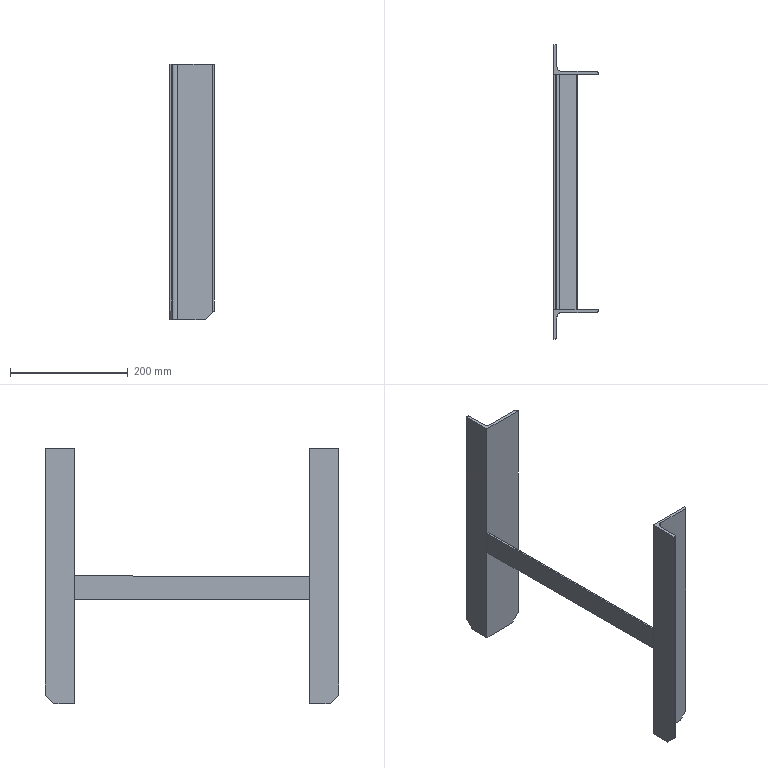Part | SolidWorks | 3 solids | 37 faces | box 75 x 500 x 435 mm | volume 652572 mm3 | plane 28 | cylinder 9 | commonest cylinder face diameters 5.333 x4 2.667 x2 16 x2 10 x1
STEP:
#1=CARTESIAN_POINT('',(75.,0.,-202.5));
#2=VERTEX_POINT('',#1);
#3=CARTESIAN_POINT('',(60.,0.,-217.5));
#4=VERTEX_POINT('',#3);
#5=CARTESIAN_POINT('',(60.,0.,-217.5));
#6=DIRECTION('',(-0.7071,0.,-0.7071));
#7=VECTOR('',#6,1000.);
#8=LINE('',#5,#7);
#9=EDGE_CURVE('',#2,#4,#8,.T.);
#10=ORIENTED_EDGE('',*,*,#9,.F.);
#11=CARTESIAN_POINT('',(75.,0.,217.5));
#12=VERTEX_POINT('',#11);
#13=CARTESIAN_POINT('',(75.,0.,-217.5));
#14=DIRECTION('',(0.,0.,1.));
#15=VECTOR('',#14,1000.);
#16=LINE('',#13,#15);
#17=EDGE_CURVE('',#2,#12,#16,.T.);
#18=ORIENTED_EDGE('',*,*,#17,.T.);
#19=CARTESIAN_POINT('',(0.,0.,217.5));
#20=VERTEX_POINT('',#19);
#21=CARTESIAN_POINT('',(0.,0.,217.5));
#22=DIRECTION('',(-1.,0.,0.));
#23=VECTOR('',#22,1000.);
#24=LINE('',#21,#23);
#25=EDGE_CURVE('',#12,#20,#24,.T.);
#26=ORIENTED_EDGE('',*,*,#25,.T.);
#27=CARTESIAN_POINT('',(0.,0.,-217.5));
#28=VERTEX_POINT('',#27);
#29=CARTESIAN_POINT('',(0.,0.,-217.5));
#30=DIRECTION('',(0.,0.,1.));
#31=VECTOR('',#30,1000.);
#32=LINE('',#29,#31);
#33=EDGE_CURVE('',#28,#20,#32,.T.);
#34=ORIENTED_EDGE('',*,*,#33,.F.);
#35=CARTESIAN_POINT('',(0.,0.,-217.5));
#36=DIRECTION('',(-1.,0.,0.));
#37=VECTOR('',#36,1000.);
#38=LINE('',#35,#37);
#39=EDGE_CURVE('',#4,#28,#38,.T.);
#40=ORIENTED_EDGE('',*,*,#39,.F.);
#41=EDGE_LOOP('',(#10,#18,#26,#34,#40));
#42=FACE_OUTER_BOUND('',#41,.T.);
#43=CARTESIAN_POINT('',(0.,0.,-217.5));
#44=DIRECTION('',(0.,1.,0.));
#45=DIRECTION('',(0.,0.,1.));
#46=AXIS2_PLACEMENT_3D('',#43,#44,#45);
#47=PLANE('',#46);
#48=ADVANCED_FACE('',(#42),#47,.F.);
#49=CARTESIAN_POINT('',(60.,5.,-217.5));
#50=VERTEX_POINT('',#49);
#51=CARTESIAN_POINT('',(60.,-617.801,-217.5));
#52=DIRECTION('',(0.,1.,0.));
#53=VECTOR('',#52,1000.);
#54=LINE('',#51,#53);
#55=EDGE_CURVE('',#4,#50,#54,.T.);
#56=ORIENTED_EDGE('',*,*,#55,.F.);
#57=ORIENTED_EDGE('',*,*,#39,.T.);
#58=CARTESIAN_POINT('',(0.,35.,-217.5));
#59=VERTEX_POINT('',#58);
#60=CARTESIAN_POINT('',(0.,50.,-217.5));
#61=DIRECTION('',(0.,1.,0.));
#62=VECTOR('',#61,1000.);
#63=LINE('',#60,#62);
#64=EDGE_CURVE('',#28,#59,#63,.T.);
#65=ORIENTED_EDGE('',*,*,#64,.T.);
#66=CARTESIAN_POINT('',(5.,35.,-217.5));
#67=VERTEX_POINT('',#66);
#68=CARTESIAN_POINT('',(-555.301,35.,-217.5));
#69=DIRECTION('',(1.,0.,0.));
#70=VECTOR('',#69,1000.);
#71=LINE('',#68,#70);
#72=EDGE_CURVE('',#59,#67,#71,.T.);
#73=ORIENTED_EDGE('',*,*,#72,.T.);
#74=CARTESIAN_POINT('',(5.,13.,-217.5));
#75=VERTEX_POINT('',#74);
#76=CARTESIAN_POINT('',(5.,13.,-217.5));
#77=DIRECTION('',(0.,-1.,0.));
#78=VECTOR('',#77,1000.);
#79=LINE('',#76,#78);
#80=EDGE_CURVE('',#67,#75,#79,.T.);
#81=ORIENTED_EDGE('',*,*,#80,.T.);
#82=CARTESIAN_POINT('',(13.,5.,-217.5));
#83=VERTEX_POINT('',#82);
#84=CARTESIAN_POINT('',(13.,13.,-217.5));
#85=DIRECTION('',(0.,0.,1.));
#86=DIRECTION('',(0.,-1.,0.));
#87=AXIS2_PLACEMENT_3D('',#84,#85,#86);
#88=CIRCLE('',#87,8.);
#89=EDGE_CURVE('',#75,#83,#88,.T.);
#90=ORIENTED_EDGE('',*,*,#89,.T.);
#91=CARTESIAN_POINT('',(72.333,5.,-217.5));
#92=DIRECTION('',(1.,0.,0.));
#93=VECTOR('',#92,1000.);
#94=LINE('',#91,#93);
#95=EDGE_CURVE('',#83,#50,#94,.T.);
#96=ORIENTED_EDGE('',*,*,#95,.T.);
#97=EDGE_LOOP('',(#56,#57,#65,#73,#81,#90,#96));
#98=FACE_OUTER_BOUND('',#97,.T.);
#99=CARTESIAN_POINT('',(72.333,2.333,-217.5));
#100=DIRECTION('',(0.,0.,1.));
#101=DIRECTION('',(0.,-1.,0.));
#102=AXIS2_PLACEMENT_3D('',#99,#100,#101);
#103=PLANE('',#102);
#104=ADVANCED_FACE('',(#98),#103,.F.);
#105=CARTESIAN_POINT('',(0.,50.,-202.5));
#106=VERTEX_POINT('',#105);
#107=CARTESIAN_POINT('',(2.333,50.,-202.5));
#108=VERTEX_POINT('',#107);
#109=CARTESIAN_POINT('',(-555.301,50.,-202.5));
#110=DIRECTION('',(1.,0.,0.));
#111=VECTOR('',#110,1000.);
#112=LINE('',#109,#111);
#113=EDGE_CURVE('',#106,#108,#112,.T.);
#114=ORIENTED_EDGE('',*,*,#113,.F.);
#115=CARTESIAN_POINT('',(0.,50.,217.5));
#116=VERTEX_POINT('',#115);
#117=CARTESIAN_POINT('',(0.,50.,-217.5));
#118=DIRECTION('',(0.,0.,1.));
#119=VECTOR('',#118,1000.);
#120=LINE('',#117,#119);
#121=EDGE_CURVE('',#106,#116,#120,.T.);
#122=ORIENTED_EDGE('',*,*,#121,.T.);
#123=CARTESIAN_POINT('',(2.333,50.,217.5));
#124=VERTEX_POINT('',#123);
#125=CARTESIAN_POINT('',(0.,50.,217.5));
#126=DIRECTION('',(1.,0.,0.));
#127=VECTOR('',#126,1000.);
#128=LINE('',#125,#127);
#129=EDGE_CURVE('',#116,#124,#128,.T.);
#130=ORIENTED_EDGE('',*,*,#129,.T.);
#131=CARTESIAN_POINT('',(2.333,50.,-217.5));
#132=DIRECTION('',(0.,0.,1.));
#133=VECTOR('',#132,1000.);
#134=LINE('',#131,#133);
#135=EDGE_CURVE('',#108,#124,#134,.T.);
#136=ORIENTED_EDGE('',*,*,#135,.F.);
#137=EDGE_LOOP('',(#114,#122,#130,#136));
#138=FACE_OUTER_BOUND('',#137,.T.);
#139=CARTESIAN_POINT('',(0.,50.,-217.5));
#140=DIRECTION('',(0.,-1.,0.));
#141=DIRECTION('',(1.,0.,0.));
#142=AXIS2_PLACEMENT_3D('',#139,#140,#141);
#143=PLANE('',#142);
#144=ADVANCED_FACE('',(#138),#143,.F.);
#145=CARTESIAN_POINT('',(5.,47.333,-205.167));
#146=VERTEX_POINT('',#145);
#147=CARTESIAN_POINT('',(2.333,50.,-202.5));
#148=CARTESIAN_POINT('',(3.895,50.,-202.5));
#149=CARTESIAN_POINT('',(5.,48.895,-203.605));
#150=CARTESIAN_POINT('',(5.,47.333,-205.167));
#151=(BOUNDED_CURVE()B_SPLINE_CURVE(3,(#147,#148,#149,#150),.UNSPECIFIED.,.F.,.F.)B_SPLINE_CURVE_WITH_KNOTS((4,4),(0.,1.571),.UNSPECIFIED.)CURVE()GEOMETRIC_REPRESENTATION_ITEM()RATIONAL_B_SPLINE_CURVE((1.,0.8047,0.8047,1.))REPRESENTATION_ITEM(''));
#152=EDGE_CURVE('',#108,#146,#151,.T.);
#153=ORIENTED_EDGE('',*,*,#152,.F.);
#154=ORIENTED_EDGE('',*,*,#135,.T.);
#155=CARTESIAN_POINT('',(5.,47.333,217.5));
#156=VERTEX_POINT('',#155);
#157=CARTESIAN_POINT('',(2.333,47.333,217.5));
#158=DIRECTION('',(0.,0.,-1.));
#159=DIRECTION('',(0.,1.,0.));
#160=AXIS2_PLACEMENT_3D('',#157,#158,#159);
#161=CIRCLE('',#160,2.667);
#162=EDGE_CURVE('',#124,#156,#161,.T.);
#163=ORIENTED_EDGE('',*,*,#162,.T.);
#164=CARTESIAN_POINT('',(5.,47.333,-217.5));
#165=DIRECTION('',(0.,0.,1.));
#166=VECTOR('',#165,1000.);
#167=LINE('',#164,#166);
#168=EDGE_CURVE('',#146,#156,#167,.T.);
#169=ORIENTED_EDGE('',*,*,#168,.F.);
#170=EDGE_LOOP('',(#153,#154,#163,#169));
#171=FACE_OUTER_BOUND('',#170,.T.);
#172=CARTESIAN_POINT('',(2.333,47.333,-217.5));
#173=DIRECTION('',(0.,0.,1.));
#174=DIRECTION('',(0.,-1.,0.));
#175=AXIS2_PLACEMENT_3D('',#172,#173,#174);
#176=CYLINDRICAL_SURFACE('',#175,2.667);
#177=ADVANCED_FACE('',(#171),#176,.T.);
#178=CARTESIAN_POINT('',(5.,24.,-228.5));
#179=DIRECTION('',(0.,-0.7071,-0.7071));
#180=VECTOR('',#179,1000.);
#181=LINE('',#178,#180);
#182=EDGE_CURVE('',#146,#67,#181,.T.);
#183=ORIENTED_EDGE('',*,*,#182,.F.);
#184=ORIENTED_EDGE('',*,*,#168,.T.);
#185=CARTESIAN_POINT('',(5.,13.,217.5));
#186=VERTEX_POINT('',#185);
#187=CARTESIAN_POINT('',(5.,13.,217.5));
#188=DIRECTION('',(0.,-1.,0.));
#189=VECTOR('',#188,1000.);
#190=LINE('',#187,#189);
#191=EDGE_CURVE('',#156,#186,#190,.T.);
#192=ORIENTED_EDGE('',*,*,#191,.T.);
#193=CARTESIAN_POINT('',(5.,13.,-217.5));
#194=DIRECTION('',(0.,0.,1.));
#195=VECTOR('',#194,1000.);
#196=LINE('',#193,#195);
#197=EDGE_CURVE('',#75,#186,#196,.T.);
#198=ORIENTED_EDGE('',*,*,#197,.F.);
#199=ORIENTED_EDGE('',*,*,#80,.F.);
#200=EDGE_LOOP('',(#183,#184,#192,#198,#199));
#201=FACE_OUTER_BOUND('',#200,.T.);
#202=CARTESIAN_POINT('',(5.,13.,-217.5));
#203=DIRECTION('',(-1.,0.,0.));
#204=DIRECTION('',(0.,-1.,0.));
#205=AXIS2_PLACEMENT_3D('',#202,#203,#204);
#206=PLANE('',#205);
#207=ADVANCED_FACE('',(#201),#206,.F.);
#208=ORIENTED_EDGE('',*,*,#121,.F.);
#209=CARTESIAN_POINT('',(0.,35.,-217.5));
#210=DIRECTION('',(0.,-0.7071,-0.7071));
#211=VECTOR('',#210,1000.);
#212=LINE('',#209,#211);
#213=EDGE_CURVE('',#106,#59,#212,.T.);
#214=ORIENTED_EDGE('',*,*,#213,.T.);
#215=ORIENTED_EDGE('',*,*,#64,.F.);
#216=ORIENTED_EDGE('',*,*,#33,.T.);
#217=CARTESIAN_POINT('',(0.,50.,217.5));
#218=DIRECTION('',(0.,1.,0.));
#219=VECTOR('',#218,1000.);
#220=LINE('',#217,#219);
#221=EDGE_CURVE('',#20,#116,#220,.T.);
#222=ORIENTED_EDGE('',*,*,#221,.T.);
#223=EDGE_LOOP('',(#208,#214,#215,#216,#222));
#224=FACE_OUTER_BOUND('',#223,.T.);
#225=CARTESIAN_POINT('',(0.,50.,-217.5));
#226=DIRECTION('',(1.,0.,0.));
#227=DIRECTION('',(0.,0.,-1.));
#228=AXIS2_PLACEMENT_3D('',#225,#226,#227);
#229=PLANE('',#228);
#230=ADVANCED_FACE('',(#224),#229,.F.);
#231=CARTESIAN_POINT('',(13.,5.,217.5));
#232=VERTEX_POINT('',#231);
#233=CARTESIAN_POINT('',(13.,13.,217.5));
#234=DIRECTION('',(0.,0.,1.));
#235=DIRECTION('',(0.,-1.,0.));
#236=AXIS2_PLACEMENT_3D('',#233,#234,#235);
#237=CIRCLE('',#236,8.);
#238=EDGE_CURVE('',#186,#232,#237,.T.);
#239=ORIENTED_EDGE('',*,*,#238,.T.);
#240=CARTESIAN_POINT('',(13.,5.,-217.5));
#241=DIRECTION('',(0.,0.,1.));
#242=VECTOR('',#241,1000.);
#243=LINE('',#240,#242);
#244=EDGE_CURVE('',#83,#232,#243,.T.);
#245=ORIENTED_EDGE('',*,*,#244,.F.);
#246=ORIENTED_EDGE('',*,*,#89,.F.);
#247=ORIENTED_EDGE('',*,*,#197,.T.);
#248=EDGE_LOOP('',(#239,#245,#246,#247));
#249=FACE_OUTER_BOUND('',#248,.T.);
#250=CARTESIAN_POINT('',(13.,13.,-217.5));
#251=DIRECTION('',(0.,0.,1.));
#252=DIRECTION('',(0.,-1.,0.));
#253=AXIS2_PLACEMENT_3D('',#250,#251,#252);
#254=CYLINDRICAL_SURFACE('',#253,8.);
#255=ADVANCED_FACE('',(#249),#254,.F.);
#256=CARTESIAN_POINT('',(72.333,5.,-205.167));
#257=VERTEX_POINT('',#256);
#258=CARTESIAN_POINT('',(72.333,5.,217.5));
#259=VERTEX_POINT('',#258);
#260=CARTESIAN_POINT('',(72.333,5.,-217.5));
#261=DIRECTION('',(0.,0.,1.));
#262=VECTOR('',#261,1000.);
#263=LINE('',#260,#262);
#264=EDGE_CURVE('',#257,#259,#263,.T.);
#265=ORIENTED_EDGE('',*,*,#264,.F.);
#266=CARTESIAN_POINT('',(66.167,5.,-211.333));
#267=DIRECTION('',(-0.7071,0.,-0.7071));
#268=VECTOR('',#267,1000.);
#269=LINE('',#266,#268);
#270=EDGE_CURVE('',#257,#50,#269,.T.);
#271=ORIENTED_EDGE('',*,*,#270,.T.);
#272=ORIENTED_EDGE('',*,*,#95,.F.);
#273=ORIENTED_EDGE('',*,*,#244,.T.);
#274=CARTESIAN_POINT('',(72.333,5.,217.5));
#275=DIRECTION('',(1.,0.,0.));
#276=VECTOR('',#275,1000.);
#277=LINE('',#274,#276);
#278=EDGE_CURVE('',#232,#259,#277,.T.);
#279=ORIENTED_EDGE('',*,*,#278,.T.);
#280=EDGE_LOOP('',(#265,#271,#272,#273,#279));
#281=FACE_OUTER_BOUND('',#280,.T.);
#282=CARTESIAN_POINT('',(72.333,5.,-217.5));
#283=DIRECTION('',(0.,-1.,0.));
#284=DIRECTION('',(0.,0.,-1.));
#285=AXIS2_PLACEMENT_3D('',#282,#283,#284);
#286=PLANE('',#285);
#287=ADVANCED_FACE('',(#281),#286,.F.);
#288=CARTESIAN_POINT('',(75.,2.333,-202.5));
#289=VERTEX_POINT('',#288);
#290=CARTESIAN_POINT('',(75.,2.333,217.5));
#291=VERTEX_POINT('',#290);
#292=CARTESIAN_POINT('',(75.,2.333,-217.5));
#293=DIRECTION('',(0.,0.,1.));
#294=VECTOR('',#293,1000.);
#295=LINE('',#292,#294);
#296=EDGE_CURVE('',#289,#291,#295,.T.);
#297=ORIENTED_EDGE('',*,*,#296,.F.);
#298=CARTESIAN_POINT('',(75.,2.333,-202.5));
#299=CARTESIAN_POINT('',(75.,3.895,-202.5));
#300=CARTESIAN_POINT('',(73.895,5.,-203.605));
#301=CARTESIAN_POINT('',(72.333,5.,-205.167));
#302=(BOUNDED_CURVE()B_SPLINE_CURVE(3,(#298,#299,#300,#301),.UNSPECIFIED.,.F.,.T.)B_SPLINE_CURVE_WITH_KNOTS((4,4),(0.,1.571),.UNSPECIFIED.)CURVE()GEOMETRIC_REPRESENTATION_ITEM()RATIONAL_B_SPLINE_CURVE((1.,0.8047,0.8047,1.))REPRESENTATION_ITEM(''));
#303=EDGE_CURVE('',#289,#257,#302,.T.);
#304=ORIENTED_EDGE('',*,*,#303,.T.);
#305=ORIENTED_EDGE('',*,*,#264,.T.);
#306=CARTESIAN_POINT('',(72.333,2.333,217.5));
#307=DIRECTION('',(0.,0.,-1.));
#308=DIRECTION('',(0.,-1.,0.));
#309=AXIS2_PLACEMENT_3D('',#306,#307,#308);
#310=CIRCLE('',#309,2.667);
#311=EDGE_CURVE('',#259,#291,#310,.T.);
#312=ORIENTED_EDGE('',*,*,#311,.T.);
#313=EDGE_LOOP('',(#297,#304,#305,#312));
#314=FACE_OUTER_BOUND('',#313,.T.);
#315=CARTESIAN_POINT('',(72.333,2.333,-217.5));
#316=DIRECTION('',(0.,0.,1.));
#317=DIRECTION('',(0.,-1.,0.));
#318=AXIS2_PLACEMENT_3D('',#315,#316,#317);
#319=CYLINDRICAL_SURFACE('',#318,2.667);
#320=ADVANCED_FACE('',(#314),#319,.T.);
#321=ORIENTED_EDGE('',*,*,#17,.F.);
#322=CARTESIAN_POINT('',(75.,-617.801,-202.5));
#323=DIRECTION('',(0.,1.,0.));
#324=VECTOR('',#323,1000.);
#325=LINE('',#322,#324);
#326=EDGE_CURVE('',#2,#289,#325,.T.);
#327=ORIENTED_EDGE('',*,*,#326,.T.);
#328=ORIENTED_EDGE('',*,*,#296,.T.);
#329=CARTESIAN_POINT('',(75.,0.,217.5));
#330=DIRECTION('',(0.,-1.,0.));
#331=VECTOR('',#330,1000.);
#332=LINE('',#329,#331);
#333=EDGE_CURVE('',#291,#12,#332,.T.);
#334=ORIENTED_EDGE('',*,*,#333,.T.);
#335=EDGE_LOOP('',(#321,#327,#328,#334));
#336=FACE_OUTER_BOUND('',#335,.T.);
#337=CARTESIAN_POINT('',(75.,0.,-217.5));
#338=DIRECTION('',(-1.,0.,0.));
#339=DIRECTION('',(0.,-1.,0.));
#340=AXIS2_PLACEMENT_3D('',#337,#338,#339);
#341=PLANE('',#340);
#342=ADVANCED_FACE('',(#336),#341,.F.);
#343=ORIENTED_EDGE('',*,*,#221,.F.);
#344=ORIENTED_EDGE('',*,*,#25,.F.);
#345=ORIENTED_EDGE('',*,*,#333,.F.);
#346=ORIENTED_EDGE('',*,*,#311,.F.);
#347=ORIENTED_EDGE('',*,*,#278,.F.);
#348=ORIENTED_EDGE('',*,*,#238,.F.);
#349=ORIENTED_EDGE('',*,*,#191,.F.);
#350=ORIENTED_EDGE('',*,*,#162,.F.);
#351=ORIENTED_EDGE('',*,*,#129,.F.);
#352=EDGE_LOOP('',(#343,#344,#345,#346,#347,#348,#349,#350,#351));
#353=FACE_OUTER_BOUND('',#352,.T.);
#354=CARTESIAN_POINT('',(72.333,2.333,217.5));
#355=DIRECTION('',(0.,0.,1.));
#356=DIRECTION('',(0.,-1.,0.));
#357=AXIS2_PLACEMENT_3D('',#354,#355,#356);
#358=PLANE('',#357);
#359=ADVANCED_FACE('',(#353),#358,.T.);
#360=ORIENTED_EDGE('',*,*,#113,.T.);
#361=ORIENTED_EDGE('',*,*,#152,.T.);
#362=ORIENTED_EDGE('',*,*,#182,.T.);
#363=ORIENTED_EDGE('',*,*,#72,.F.);
#364=ORIENTED_EDGE('',*,*,#213,.F.);
#365=EDGE_LOOP('',(#360,#361,#362,#363,#364));
#366=FACE_OUTER_BOUND('',#365,.T.);
#367=CARTESIAN_POINT('',(-555.301,35.,-217.5));
#368=DIRECTION('',(0.,0.7071,-0.7071));
#369=DIRECTION('',(0.,0.7071,0.7071));
#370=AXIS2_PLACEMENT_3D('',#367,#368,#369);
#371=PLANE('',#370);
#372=ADVANCED_FACE('',(#366),#371,.T.);
#373=ORIENTED_EDGE('',*,*,#270,.F.);
#374=ORIENTED_EDGE('',*,*,#303,.F.);
#375=ORIENTED_EDGE('',*,*,#326,.F.);
#376=ORIENTED_EDGE('',*,*,#9,.T.);
#377=ORIENTED_EDGE('',*,*,#55,.T.);
#378=EDGE_LOOP('',(#373,#374,#375,#376,#377));
#379=FACE_OUTER_BOUND('',#378,.T.);
#380=CARTESIAN_POINT('',(60.,-617.801,-217.5));
#381=DIRECTION('',(-0.7071,0.,0.7071));
#382=DIRECTION('',(0.7071,0.,0.7071));
#383=AXIS2_PLACEMENT_3D('',#380,#381,#382);
#384=PLANE('',#383);
#385=ADVANCED_FACE('',(#379),#384,.F.);
#386=CLOSED_SHELL('',(#48,#104,#144,#177,#207,#230,#255,#287,#320,#342,#359,#372,#385));
#387=MANIFOLD_SOLID_BREP('',#386);
#388=CARTESIAN_POINT('',(75.,-400.,-202.5));
#389=VERTEX_POINT('',#388);
#390=CARTESIAN_POINT('',(60.,-400.,-217.5));
#391=VERTEX_POINT('',#390);
#392=CARTESIAN_POINT('',(60.,-400.,-217.5));
#393=DIRECTION('',(-0.7071,0.,-0.7071));
#394=VECTOR('',#393,1000.);
#395=LINE('',#392,#394);
#396=EDGE_CURVE('',#389,#391,#395,.T.);
#397=ORIENTED_EDGE('',*,*,#396,.T.);
#398=CARTESIAN_POINT('',(0.,-400.,-217.5));
#399=VERTEX_POINT('',#398);
#400=CARTESIAN_POINT('',(0.,-400.,-217.5));
#401=DIRECTION('',(-1.,0.,0.));
#402=VECTOR('',#401,1000.);
#403=LINE('',#400,#402);
#404=EDGE_CURVE('',#391,#399,#403,.T.);
#405=ORIENTED_EDGE('',*,*,#404,.T.);
#406=CARTESIAN_POINT('',(0.,-400.,217.5));
#407=VERTEX_POINT('',#406);
#408=CARTESIAN_POINT('',(0.,-400.,-217.5));
#409=DIRECTION('',(0.,0.,1.));
#410=VECTOR('',#409,1000.);
#411=LINE('',#408,#410);
#412=EDGE_CURVE('',#399,#407,#411,.T.);
#413=ORIENTED_EDGE('',*,*,#412,.T.);
#414=CARTESIAN_POINT('',(75.,-400.,217.5));
#415=VERTEX_POINT('',#414);
#416=CARTESIAN_POINT('',(0.,-400.,217.5));
#417=DIRECTION('',(-1.,0.,0.));
#418=VECTOR('',#417,1000.);
#419=LINE('',#416,#418);
#420=EDGE_CURVE('',#415,#407,#419,.T.);
#421=ORIENTED_EDGE('',*,*,#420,.F.);
#422=CARTESIAN_POINT('',(75.,-400.,-217.5));
#423=DIRECTION('',(0.,0.,1.));
#424=VECTOR('',#423,1000.);
#425=LINE('',#422,#424);
#426=EDGE_CURVE('',#389,#415,#425,.T.);
#427=ORIENTED_EDGE('',*,*,#426,.F.);
#428=EDGE_LOOP('',(#397,#405,#413,#421,#427));
#429=FACE_OUTER_BOUND('',#428,.T.);
#430=CARTESIAN_POINT('',(0.,-400.,-217.5));
#431=DIRECTION('',(0.,-1.,0.));
#432=DIRECTION('',(0.,0.,1.));
#433=AXIS2_PLACEMENT_3D('',#430,#431,#432);
#434=PLANE('',#433);
#435=ADVANCED_FACE('',(#429),#434,.F.);
#436=CARTESIAN_POINT('',(60.,-405.,-217.5));
#437=VERTEX_POINT('',#436);
#438=CARTESIAN_POINT('',(60.,217.801,-217.5));
#439=DIRECTION('',(0.,-1.,0.));
#440=VECTOR('',#439,1000.);
#441=LINE('',#438,#440);
#442=EDGE_CURVE('',#391,#437,#441,.T.);
#443=ORIENTED_EDGE('',*,*,#442,.T.);
#444=CARTESIAN_POINT('',(13.,-405.,-217.5));
#445=VERTEX_POINT('',#444);
#446=CARTESIAN_POINT('',(72.333,-405.,-217.5));
#447=DIRECTION('',(1.,0.,0.));
#448=VECTOR('',#447,1000.);
#449=LINE('',#446,#448);
#450=EDGE_CURVE('',#445,#437,#449,.T.);
#451=ORIENTED_EDGE('',*,*,#450,.F.);
#452=CARTESIAN_POINT('',(5.,-413.,-217.5));
#453=VERTEX_POINT('',#452);
#454=CARTESIAN_POINT('',(13.,-413.,-217.5));
#455=DIRECTION('',(0.,0.,-1.));
#456=DIRECTION('',(0.,1.,0.));
#457=AXIS2_PLACEMENT_3D('',#454,#455,#456);
#458=CIRCLE('',#457,8.);
#459=EDGE_CURVE('',#453,#445,#458,.T.);
#460=ORIENTED_EDGE('',*,*,#459,.F.);
#461=CARTESIAN_POINT('',(5.,-435.,-217.5));
#462=VERTEX_POINT('',#461);
#463=CARTESIAN_POINT('',(5.,-413.,-217.5));
#464=DIRECTION('',(0.,1.,0.));
#465=VECTOR('',#464,1000.);
#466=LINE('',#463,#465);
#467=EDGE_CURVE('',#462,#453,#466,.T.);
#468=ORIENTED_EDGE('',*,*,#467,.F.);
#469=CARTESIAN_POINT('',(0.,-435.,-217.5));
#470=VERTEX_POINT('',#469);
#471=CARTESIAN_POINT('',(-555.301,-435.,-217.5));
#472=DIRECTION('',(1.,0.,0.));
#473=VECTOR('',#472,1000.);
#474=LINE('',#471,#473);
#475=EDGE_CURVE('',#470,#462,#474,.T.);
#476=ORIENTED_EDGE('',*,*,#475,.F.);
#477=CARTESIAN_POINT('',(0.,-450.,-217.5));
#478=DIRECTION('',(0.,-1.,0.));
#479=VECTOR('',#478,1000.);
#480=LINE('',#477,#479);
#481=EDGE_CURVE('',#399,#470,#480,.T.);
#482=ORIENTED_EDGE('',*,*,#481,.F.);
#483=ORIENTED_EDGE('',*,*,#404,.F.);
#484=EDGE_LOOP('',(#443,#451,#460,#468,#476,#482,#483));
#485=FACE_OUTER_BOUND('',#484,.T.);
#486=CARTESIAN_POINT('',(72.333,-402.333,-217.5));
#487=DIRECTION('',(0.,0.,1.));
#488=DIRECTION('',(0.,1.,0.));
#489=AXIS2_PLACEMENT_3D('',#486,#487,#488);
#490=PLANE('',#489);
#491=ADVANCED_FACE('',(#485),#490,.F.);
#492=CARTESIAN_POINT('',(0.,-450.,-202.5));
#493=VERTEX_POINT('',#492);
#494=CARTESIAN_POINT('',(2.333,-450.,-202.5));
#495=VERTEX_POINT('',#494);
#496=CARTESIAN_POINT('',(-555.301,-450.,-202.5));
#497=DIRECTION('',(1.,0.,0.));
#498=VECTOR('',#497,1000.);
#499=LINE('',#496,#498);
#500=EDGE_CURVE('',#493,#495,#499,.T.);
#501=ORIENTED_EDGE('',*,*,#500,.T.);
#502=CARTESIAN_POINT('',(2.333,-450.,217.5));
#503=VERTEX_POINT('',#502);
#504=CARTESIAN_POINT('',(2.333,-450.,-217.5));
#505=DIRECTION('',(0.,0.,1.));
#506=VECTOR('',#505,1000.);
#507=LINE('',#504,#506);
#508=EDGE_CURVE('',#495,#503,#507,.T.);
#509=ORIENTED_EDGE('',*,*,#508,.T.);
#510=CARTESIAN_POINT('',(0.,-450.,217.5));
#511=VERTEX_POINT('',#510);
#512=CARTESIAN_POINT('',(0.,-450.,217.5));
#513=DIRECTION('',(1.,0.,0.));
#514=VECTOR('',#513,1000.);
#515=LINE('',#512,#514);
#516=EDGE_CURVE('',#511,#503,#515,.T.);
#517=ORIENTED_EDGE('',*,*,#516,.F.);
#518=CARTESIAN_POINT('',(0.,-450.,-217.5));
#519=DIRECTION('',(0.,0.,1.));
#520=VECTOR('',#519,1000.);
#521=LINE('',#518,#520);
#522=EDGE_CURVE('',#493,#511,#521,.T.);
#523=ORIENTED_EDGE('',*,*,#522,.F.);
#524=EDGE_LOOP('',(#501,#509,#517,#523));
#525=FACE_OUTER_BOUND('',#524,.T.);
#526=CARTESIAN_POINT('',(0.,-450.,-217.5));
#527=DIRECTION('',(0.,1.,0.));
#528=DIRECTION('',(1.,0.,0.));
#529=AXIS2_PLACEMENT_3D('',#526,#527,#528);
#530=PLANE('',#529);
#531=ADVANCED_FACE('',(#525),#530,.F.);
#532=CARTESIAN_POINT('',(5.,-447.333,-205.167));
#533=VERTEX_POINT('',#532);
#534=CARTESIAN_POINT('',(2.333,-450.,-202.5));
#535=CARTESIAN_POINT('',(3.895,-450.,-202.5));
#536=CARTESIAN_POINT('',(5.,-448.895,-203.605));
#537=CARTESIAN_POINT('',(5.,-447.333,-205.167));
#538=(BOUNDED_CURVE()B_SPLINE_CURVE(3,(#534,#535,#536,#537),.UNSPECIFIED.,.F.,.T.)B_SPLINE_CURVE_WITH_KNOTS((4,4),(0.,1.571),.UNSPECIFIED.)CURVE()GEOMETRIC_REPRESENTATION_ITEM()RATIONAL_B_SPLINE_CURVE((1.,0.8047,0.8047,1.))REPRESENTATION_ITEM(''));
#539=EDGE_CURVE('',#495,#533,#538,.T.);
#540=ORIENTED_EDGE('',*,*,#539,.T.);
#541=CARTESIAN_POINT('',(5.,-447.333,217.5));
#542=VERTEX_POINT('',#541);
#543=CARTESIAN_POINT('',(5.,-447.333,-217.5));
#544=DIRECTION('',(0.,0.,1.));
#545=VECTOR('',#544,1000.);
#546=LINE('',#543,#545);
#547=EDGE_CURVE('',#533,#542,#546,.T.);
#548=ORIENTED_EDGE('',*,*,#547,.T.);
#549=CARTESIAN_POINT('',(2.333,-447.333,217.5));
#550=DIRECTION('',(0.,0.,1.));
#551=DIRECTION('',(0.,-1.,0.));
#552=AXIS2_PLACEMENT_3D('',#549,#550,#551);
#553=CIRCLE('',#552,2.667);
#554=EDGE_CURVE('',#503,#542,#553,.T.);
#555=ORIENTED_EDGE('',*,*,#554,.F.);
#556=ORIENTED_EDGE('',*,*,#508,.F.);
#557=EDGE_LOOP('',(#540,#548,#555,#556));
#558=FACE_OUTER_BOUND('',#557,.T.);
#559=CARTESIAN_POINT('',(2.333,-447.333,-217.5));
#560=DIRECTION('',(0.,0.,1.));
#561=DIRECTION('',(0.,1.,0.));
#562=AXIS2_PLACEMENT_3D('',#559,#560,#561);
#563=CYLINDRICAL_SURFACE('',#562,2.667);
#564=ADVANCED_FACE('',(#558),#563,.T.);
#565=CARTESIAN_POINT('',(5.,-424.,-228.5));
#566=DIRECTION('',(0.,0.7071,-0.7071));
#567=VECTOR('',#566,1000.);
#568=LINE('',#565,#567);
#569=EDGE_CURVE('',#533,#462,#568,.T.);
#570=ORIENTED_EDGE('',*,*,#569,.T.);
#571=ORIENTED_EDGE('',*,*,#467,.T.);
#572=CARTESIAN_POINT('',(5.,-413.,217.5));
#573=VERTEX_POINT('',#572);
#574=CARTESIAN_POINT('',(5.,-413.,-217.5));
#575=DIRECTION('',(0.,0.,1.));
#576=VECTOR('',#575,1000.);
#577=LINE('',#574,#576);
#578=EDGE_CURVE('',#453,#573,#577,.T.);
#579=ORIENTED_EDGE('',*,*,#578,.T.);
#580=CARTESIAN_POINT('',(5.,-413.,217.5));
#581=DIRECTION('',(0.,1.,0.));
#582=VECTOR('',#581,1000.);
#583=LINE('',#580,#582);
#584=EDGE_CURVE('',#542,#573,#583,.T.);
#585=ORIENTED_EDGE('',*,*,#584,.F.);
#586=ORIENTED_EDGE('',*,*,#547,.F.);
#587=EDGE_LOOP('',(#570,#571,#579,#585,#586));
#588=FACE_OUTER_BOUND('',#587,.T.);
#589=CARTESIAN_POINT('',(5.,-413.,-217.5));
#590=DIRECTION('',(-1.,0.,0.));
#591=DIRECTION('',(0.,1.,0.));
#592=AXIS2_PLACEMENT_3D('',#589,#590,#591);
#593=PLANE('',#592);
#594=ADVANCED_FACE('',(#588),#593,.F.);
#595=ORIENTED_EDGE('',*,*,#522,.T.);
#596=CARTESIAN_POINT('',(0.,-450.,217.5));
#597=DIRECTION('',(0.,-1.,0.));
#598=VECTOR('',#597,1000.);
#599=LINE('',#596,#598);
#600=EDGE_CURVE('',#407,#511,#599,.T.);
#601=ORIENTED_EDGE('',*,*,#600,.F.);
#602=ORIENTED_EDGE('',*,*,#412,.F.);
#603=ORIENTED_EDGE('',*,*,#481,.T.);
#604=CARTESIAN_POINT('',(0.,-435.,-217.5));
#605=DIRECTION('',(0.,0.7071,-0.7071));
#606=VECTOR('',#605,1000.);
#607=LINE('',#604,#606);
#608=EDGE_CURVE('',#493,#470,#607,.T.);
#609=ORIENTED_EDGE('',*,*,#608,.F.);
#610=EDGE_LOOP('',(#595,#601,#602,#603,#609));
#611=FACE_OUTER_BOUND('',#610,.T.);
#612=CARTESIAN_POINT('',(0.,-450.,-217.5));
#613=DIRECTION('',(1.,0.,0.));
#614=DIRECTION('',(0.,0.,-1.));
#615=AXIS2_PLACEMENT_3D('',#612,#613,#614);
#616=PLANE('',#615);
#617=ADVANCED_FACE('',(#611),#616,.F.);
#618=CARTESIAN_POINT('',(13.,-405.,217.5));
#619=VERTEX_POINT('',#618);
#620=CARTESIAN_POINT('',(13.,-413.,217.5));
#621=DIRECTION('',(0.,0.,-1.));
#622=DIRECTION('',(0.,1.,0.));
#623=AXIS2_PLACEMENT_3D('',#620,#621,#622);
#624=CIRCLE('',#623,8.);
#625=EDGE_CURVE('',#573,#619,#624,.T.);
#626=ORIENTED_EDGE('',*,*,#625,.F.);
#627=ORIENTED_EDGE('',*,*,#578,.F.);
#628=ORIENTED_EDGE('',*,*,#459,.T.);
#629=CARTESIAN_POINT('',(13.,-405.,-217.5));
#630=DIRECTION('',(0.,0.,1.));
#631=VECTOR('',#630,1000.);
#632=LINE('',#629,#631);
#633=EDGE_CURVE('',#445,#619,#632,.T.);
#634=ORIENTED_EDGE('',*,*,#633,.T.);
#635=EDGE_LOOP('',(#626,#627,#628,#634));
#636=FACE_OUTER_BOUND('',#635,.T.);
#637=CARTESIAN_POINT('',(13.,-413.,-217.5));
#638=DIRECTION('',(0.,0.,1.));
#639=DIRECTION('',(0.,1.,0.));
#640=AXIS2_PLACEMENT_3D('',#637,#638,#639);
#641=CYLINDRICAL_SURFACE('',#640,8.);
#642=ADVANCED_FACE('',(#636),#641,.F.);
#643=CARTESIAN_POINT('',(72.333,-405.,-205.167));
#644=VERTEX_POINT('',#643);
#645=CARTESIAN_POINT('',(72.333,-405.,217.5));
#646=VERTEX_POINT('',#645);
#647=CARTESIAN_POINT('',(72.333,-405.,-217.5));
#648=DIRECTION('',(0.,0.,1.));
#649=VECTOR('',#648,1000.);
#650=LINE('',#647,#649);
#651=EDGE_CURVE('',#644,#646,#650,.T.);
#652=ORIENTED_EDGE('',*,*,#651,.T.);
#653=CARTESIAN_POINT('',(72.333,-405.,217.5));
#654=DIRECTION('',(1.,0.,0.));
#655=VECTOR('',#654,1000.);
#656=LINE('',#653,#655);
#657=EDGE_CURVE('',#619,#646,#656,.T.);
#658=ORIENTED_EDGE('',*,*,#657,.F.);
#659=ORIENTED_EDGE('',*,*,#633,.F.);
#660=ORIENTED_EDGE('',*,*,#450,.T.);
#661=CARTESIAN_POINT('',(66.167,-405.,-211.333));
#662=DIRECTION('',(-0.7071,0.,-0.7071));
#663=VECTOR('',#662,1000.);
#664=LINE('',#661,#663);
#665=EDGE_CURVE('',#644,#437,#664,.T.);
#666=ORIENTED_EDGE('',*,*,#665,.F.);
#667=EDGE_LOOP('',(#652,#658,#659,#660,#666));
#668=FACE_OUTER_BOUND('',#667,.T.);
#669=CARTESIAN_POINT('',(72.333,-405.,-217.5));
#670=DIRECTION('',(0.,1.,0.));
#671=DIRECTION('',(0.,0.,-1.));
#672=AXIS2_PLACEMENT_3D('',#669,#670,#671);
#673=PLANE('',#672);
#674=ADVANCED_FACE('',(#668),#673,.F.);
#675=CARTESIAN_POINT('',(75.,-402.333,-202.5));
#676=VERTEX_POINT('',#675);
#677=CARTESIAN_POINT('',(75.,-402.333,217.5));
#678=VERTEX_POINT('',#677);
#679=CARTESIAN_POINT('',(75.,-402.333,-217.5));
#680=DIRECTION('',(0.,0.,1.));
#681=VECTOR('',#680,1000.);
#682=LINE('',#679,#681);
#683=EDGE_CURVE('',#676,#678,#682,.T.);
#684=ORIENTED_EDGE('',*,*,#683,.T.);
#685=CARTESIAN_POINT('',(72.333,-402.333,217.5));
#686=DIRECTION('',(0.,0.,1.));
#687=DIRECTION('',(0.,1.,0.));
#688=AXIS2_PLACEMENT_3D('',#685,#686,#687);
#689=CIRCLE('',#688,2.667);
#690=EDGE_CURVE('',#646,#678,#689,.T.);
#691=ORIENTED_EDGE('',*,*,#690,.F.);
#692=ORIENTED_EDGE('',*,*,#651,.F.);
#693=CARTESIAN_POINT('',(75.,-402.333,-202.5));
#694=CARTESIAN_POINT('',(75.,-403.895,-202.5));
#695=CARTESIAN_POINT('',(73.895,-405.,-203.605));
#696=CARTESIAN_POINT('',(72.333,-405.,-205.167));
#697=(BOUNDED_CURVE()B_SPLINE_CURVE(3,(#693,#694,#695,#696),.UNSPECIFIED.,.F.,.F.)B_SPLINE_CURVE_WITH_KNOTS((4,4),(0.,1.571),.UNSPECIFIED.)CURVE()GEOMETRIC_REPRESENTATION_ITEM()RATIONAL_B_SPLINE_CURVE((1.,0.8047,0.8047,1.))REPRESENTATION_ITEM(''));
#698=EDGE_CURVE('',#676,#644,#697,.T.);
#699=ORIENTED_EDGE('',*,*,#698,.F.);
#700=EDGE_LOOP('',(#684,#691,#692,#699));
#701=FACE_OUTER_BOUND('',#700,.T.);
#702=CARTESIAN_POINT('',(72.333,-402.333,-217.5));
#703=DIRECTION('',(0.,0.,1.));
#704=DIRECTION('',(0.,1.,0.));
#705=AXIS2_PLACEMENT_3D('',#702,#703,#704);
#706=CYLINDRICAL_SURFACE('',#705,2.667);
#707=ADVANCED_FACE('',(#701),#706,.T.);
#708=ORIENTED_EDGE('',*,*,#426,.T.);
#709=CARTESIAN_POINT('',(75.,-400.,217.5));
#710=DIRECTION('',(0.,1.,0.));
#711=VECTOR('',#710,1000.);
#712=LINE('',#709,#711);
#713=EDGE_CURVE('',#678,#415,#712,.T.);
#714=ORIENTED_EDGE('',*,*,#713,.F.);
#715=ORIENTED_EDGE('',*,*,#683,.F.);
#716=CARTESIAN_POINT('',(75.,217.801,-202.5));
#717=DIRECTION('',(0.,-1.,0.));
#718=VECTOR('',#717,1000.);
#719=LINE('',#716,#718);
#720=EDGE_CURVE('',#389,#676,#719,.T.);
#721=ORIENTED_EDGE('',*,*,#720,.F.);
#722=EDGE_LOOP('',(#708,#714,#715,#721));
#723=FACE_OUTER_BOUND('',#722,.T.);
#724=CARTESIAN_POINT('',(75.,-400.,-217.5));
#725=DIRECTION('',(-1.,0.,0.));
#726=DIRECTION('',(0.,1.,0.));
#727=AXIS2_PLACEMENT_3D('',#724,#725,#726);
#728=PLANE('',#727);
#729=ADVANCED_FACE('',(#723),#728,.F.);
#730=ORIENTED_EDGE('',*,*,#600,.T.);
#731=ORIENTED_EDGE('',*,*,#516,.T.);
#732=ORIENTED_EDGE('',*,*,#554,.T.);
#733=ORIENTED_EDGE('',*,*,#584,.T.);
#734=ORIENTED_EDGE('',*,*,#625,.T.);
#735=ORIENTED_EDGE('',*,*,#657,.T.);
#736=ORIENTED_EDGE('',*,*,#690,.T.);
#737=ORIENTED_EDGE('',*,*,#713,.T.);
#738=ORIENTED_EDGE('',*,*,#420,.T.);
#739=EDGE_LOOP('',(#730,#731,#732,#733,#734,#735,#736,#737,#738));
#740=FACE_OUTER_BOUND('',#739,.T.);
#741=CARTESIAN_POINT('',(72.333,-402.333,217.5));
#742=DIRECTION('',(0.,0.,1.));
#743=DIRECTION('',(0.,1.,0.));
#744=AXIS2_PLACEMENT_3D('',#741,#742,#743);
#745=PLANE('',#744);
#746=ADVANCED_FACE('',(#740),#745,.T.);
#747=ORIENTED_EDGE('',*,*,#500,.F.);
#748=ORIENTED_EDGE('',*,*,#608,.T.);
#749=ORIENTED_EDGE('',*,*,#475,.T.);
#750=ORIENTED_EDGE('',*,*,#569,.F.);
#751=ORIENTED_EDGE('',*,*,#539,.F.);
#752=EDGE_LOOP('',(#747,#748,#749,#750,#751));
#753=FACE_OUTER_BOUND('',#752,.T.);
#754=CARTESIAN_POINT('',(-555.301,-435.,-217.5));
#755=DIRECTION('',(0.,-0.7071,-0.7071));
#756=DIRECTION('',(0.,-0.7071,0.7071));
#757=AXIS2_PLACEMENT_3D('',#754,#755,#756);
#758=PLANE('',#757);
#759=ADVANCED_FACE('',(#753),#758,.T.);
#760=ORIENTED_EDGE('',*,*,#665,.T.);
#761=ORIENTED_EDGE('',*,*,#442,.F.);
#762=ORIENTED_EDGE('',*,*,#396,.F.);
#763=ORIENTED_EDGE('',*,*,#720,.T.);
#764=ORIENTED_EDGE('',*,*,#698,.T.);
#765=EDGE_LOOP('',(#760,#761,#762,#763,#764));
#766=FACE_OUTER_BOUND('',#765,.T.);
#767=CARTESIAN_POINT('',(60.,217.801,-217.5));
#768=DIRECTION('',(-0.7071,0.,0.7071));
#769=DIRECTION('',(0.7071,0.,0.7071));
#770=AXIS2_PLACEMENT_3D('',#767,#768,#769);
#771=PLANE('',#770);
#772=ADVANCED_FACE('',(#766),#771,.F.);
#773=CLOSED_SHELL('',(#435,#491,#531,#564,#594,#617,#642,#674,#707,#729,#746,#759,#772));
#774=MANIFOLD_SOLID_BREP('',#773);
#775=CARTESIAN_POINT('',(0.,0.,-40.));
#776=VERTEX_POINT('',#775);
#777=CARTESIAN_POINT('',(0.,0.,0.));
#778=VERTEX_POINT('',#777);
#779=CARTESIAN_POINT('',(0.,0.,0.));
#780=DIRECTION('',(0.,0.,1.));
#781=VECTOR('',#780,1000.);
#782=LINE('',#779,#781);
#783=EDGE_CURVE('',#776,#778,#782,.T.);
#784=ORIENTED_EDGE('',*,*,#783,.F.);
#785=CARTESIAN_POINT('',(0.,-400.,-40.));
#786=VERTEX_POINT('',#785);
#787=CARTESIAN_POINT('',(0.,-400.,-40.));
#788=DIRECTION('',(0.,1.,0.));
#789=VECTOR('',#788,1000.);
#790=LINE('',#787,#789);
#791=EDGE_CURVE('',#786,#776,#790,.T.);
#792=ORIENTED_EDGE('',*,*,#791,.F.);
#793=CARTESIAN_POINT('',(0.,-400.,0.));
#794=VERTEX_POINT('',#793);
#795=CARTESIAN_POINT('',(0.,-400.,0.));
#796=DIRECTION('',(0.,0.,1.));
#797=VECTOR('',#796,1000.);
#798=LINE('',#795,#797);
#799=EDGE_CURVE('',#786,#794,#798,.T.);
#800=ORIENTED_EDGE('',*,*,#799,.T.);
#801=CARTESIAN_POINT('',(0.,-400.,0.));
#802=DIRECTION('',(0.,1.,0.));
#803=VECTOR('',#802,1000.);
#804=LINE('',#801,#803);
#805=EDGE_CURVE('',#794,#778,#804,.T.);
#806=ORIENTED_EDGE('',*,*,#805,.T.);
#807=EDGE_LOOP('',(#784,#792,#800,#806));
#808=FACE_OUTER_BOUND('',#807,.T.);
#809=CARTESIAN_POINT('',(0.,-400.,0.));
#810=DIRECTION('',(-1.,0.,0.));
#811=DIRECTION('',(0.,0.,1.));
#812=AXIS2_PLACEMENT_3D('',#809,#810,#811);
#813=PLANE('',#812);
#814=ADVANCED_FACE('',(#808),#813,.T.);
#815=CARTESIAN_POINT('',(40.,0.,-40.));
#816=VERTEX_POINT('',#815);
#817=CARTESIAN_POINT('',(0.,0.,-40.));
#818=DIRECTION('',(-1.,0.,0.));
#819=VECTOR('',#818,1000.);
#820=LINE('',#817,#819);
#821=EDGE_CURVE('',#816,#776,#820,.T.);
#822=ORIENTED_EDGE('',*,*,#821,.F.);
#823=CARTESIAN_POINT('',(40.,-400.,-40.));
#824=VERTEX_POINT('',#823);
#825=CARTESIAN_POINT('',(40.,-400.,-40.));
#826=DIRECTION('',(0.,1.,0.));
#827=VECTOR('',#826,1000.);
#828=LINE('',#825,#827);
#829=EDGE_CURVE('',#824,#816,#828,.T.);
#830=ORIENTED_EDGE('',*,*,#829,.F.);
#831=CARTESIAN_POINT('',(0.,-400.,-40.));
#832=DIRECTION('',(-1.,0.,0.));
#833=VECTOR('',#832,1000.);
#834=LINE('',#831,#833);
#835=EDGE_CURVE('',#824,#786,#834,.T.);
#836=ORIENTED_EDGE('',*,*,#835,.T.);
#837=ORIENTED_EDGE('',*,*,#791,.T.);
#838=EDGE_LOOP('',(#822,#830,#836,#837));
#839=FACE_OUTER_BOUND('',#838,.T.);
#840=CARTESIAN_POINT('',(0.,-400.,-40.));
#841=DIRECTION('',(0.,0.,-1.));
#842=DIRECTION('',(0.,1.,0.));
#843=AXIS2_PLACEMENT_3D('',#840,#841,#842);
#844=PLANE('',#843);
#845=ADVANCED_FACE('',(#839),#844,.T.);
#846=CARTESIAN_POINT('',(40.,0.,-37.333));
#847=VERTEX_POINT('',#846);
#848=CARTESIAN_POINT('',(40.,0.,-40.));
#849=DIRECTION('',(0.,0.,-1.));
#850=VECTOR('',#849,1000.);
#851=LINE('',#848,#850);
#852=EDGE_CURVE('',#847,#816,#851,.T.);
#853=ORIENTED_EDGE('',*,*,#852,.F.);
#854=CARTESIAN_POINT('',(40.,-400.,-37.333));
#855=VERTEX_POINT('',#854);
#856=CARTESIAN_POINT('',(40.,-400.,-37.333));
#857=DIRECTION('',(0.,1.,0.));
#858=VECTOR('',#857,1000.);
#859=LINE('',#856,#858);
#860=EDGE_CURVE('',#855,#847,#859,.T.);
#861=ORIENTED_EDGE('',*,*,#860,.F.);
#862=CARTESIAN_POINT('',(40.,-400.,-40.));
#863=DIRECTION('',(0.,0.,-1.));
#864=VECTOR('',#863,1000.);
#865=LINE('',#862,#864);
#866=EDGE_CURVE('',#855,#824,#865,.T.);
#867=ORIENTED_EDGE('',*,*,#866,.T.);
#868=ORIENTED_EDGE('',*,*,#829,.T.);
#869=EDGE_LOOP('',(#853,#861,#867,#868));
#870=FACE_OUTER_BOUND('',#869,.T.);
#871=CARTESIAN_POINT('',(40.,-400.,-40.));
#872=DIRECTION('',(1.,0.,0.));
#873=DIRECTION('',(0.,0.,-1.));
#874=AXIS2_PLACEMENT_3D('',#871,#872,#873);
#875=PLANE('',#874);
#876=ADVANCED_FACE('',(#870),#875,.T.);
#877=CARTESIAN_POINT('',(38.667,0.,-36.));
#878=VERTEX_POINT('',#877);
#879=CARTESIAN_POINT('',(38.667,0.,-37.333));
#880=DIRECTION('',(0.,1.,0.));
#881=DIRECTION('',(-1.,0.,0.));
#882=AXIS2_PLACEMENT_3D('',#879,#880,#881);
#883=CIRCLE('',#882,1.333);
#884=EDGE_CURVE('',#878,#847,#883,.T.);
#885=ORIENTED_EDGE('',*,*,#884,.F.);
#886=CARTESIAN_POINT('',(38.667,-400.,-36.));
#887=VERTEX_POINT('',#886);
#888=CARTESIAN_POINT('',(38.667,-400.,-36.));
#889=DIRECTION('',(0.,1.,0.));
#890=VECTOR('',#889,1000.);
#891=LINE('',#888,#890);
#892=EDGE_CURVE('',#887,#878,#891,.T.);
#893=ORIENTED_EDGE('',*,*,#892,.F.);
#894=CARTESIAN_POINT('',(38.667,-400.,-37.333));
#895=DIRECTION('',(0.,1.,0.));
#896=DIRECTION('',(-1.,0.,0.));
#897=AXIS2_PLACEMENT_3D('',#894,#895,#896);
#898=CIRCLE('',#897,1.333);
#899=EDGE_CURVE('',#887,#855,#898,.T.);
#900=ORIENTED_EDGE('',*,*,#899,.T.);
#901=ORIENTED_EDGE('',*,*,#860,.T.);
#902=EDGE_LOOP('',(#885,#893,#900,#901));
#903=FACE_OUTER_BOUND('',#902,.T.);
#904=CARTESIAN_POINT('',(38.667,-400.,-37.333));
#905=DIRECTION('',(0.,1.,0.));
#906=DIRECTION('',(0.,0.,1.));
#907=AXIS2_PLACEMENT_3D('',#904,#905,#906);
#908=CYLINDRICAL_SURFACE('',#907,1.333);
#909=ADVANCED_FACE('',(#903),#908,.T.);
#910=CARTESIAN_POINT('',(9.,0.,-36.));
#911=VERTEX_POINT('',#910);
#912=CARTESIAN_POINT('',(38.667,0.,-36.));
#913=DIRECTION('',(1.,0.,0.));
#914=VECTOR('',#913,1000.);
#915=LINE('',#912,#914);
#916=EDGE_CURVE('',#911,#878,#915,.T.);
#917=ORIENTED_EDGE('',*,*,#916,.F.);
#918=CARTESIAN_POINT('',(9.,-400.,-36.));
#919=VERTEX_POINT('',#918);
#920=CARTESIAN_POINT('',(9.,-400.,-36.));
#921=DIRECTION('',(0.,1.,0.));
#922=VECTOR('',#921,1000.);
#923=LINE('',#920,#922);
#924=EDGE_CURVE('',#919,#911,#923,.T.);
#925=ORIENTED_EDGE('',*,*,#924,.F.);
#926=CARTESIAN_POINT('',(38.667,-400.,-36.));
#927=DIRECTION('',(1.,0.,0.));
#928=VECTOR('',#927,1000.);
#929=LINE('',#926,#928);
#930=EDGE_CURVE('',#919,#887,#929,.T.);
#931=ORIENTED_EDGE('',*,*,#930,.T.);
#932=ORIENTED_EDGE('',*,*,#892,.T.);
#933=EDGE_LOOP('',(#917,#925,#931,#932));
#934=FACE_OUTER_BOUND('',#933,.T.);
#935=CARTESIAN_POINT('',(38.667,-400.,-36.));
#936=DIRECTION('',(0.,0.,1.));
#937=DIRECTION('',(0.,-1.,0.));
#938=AXIS2_PLACEMENT_3D('',#935,#936,#937);
#939=PLANE('',#938);
#940=ADVANCED_FACE('',(#934),#939,.T.);
#941=CARTESIAN_POINT('',(4.,0.,-31.));
#942=VERTEX_POINT('',#941);
#943=CARTESIAN_POINT('',(9.,0.,-31.));
#944=DIRECTION('',(0.,-1.,0.));
#945=DIRECTION('',(-1.,0.,0.));
#946=AXIS2_PLACEMENT_3D('',#943,#944,#945);
#947=CIRCLE('',#946,5.);
#948=EDGE_CURVE('',#942,#911,#947,.T.);
#949=ORIENTED_EDGE('',*,*,#948,.F.);
#950=CARTESIAN_POINT('',(4.,-400.,-31.));
#951=VERTEX_POINT('',#950);
#952=CARTESIAN_POINT('',(4.,-400.,-31.));
#953=DIRECTION('',(0.,1.,0.));
#954=VECTOR('',#953,1000.);
#955=LINE('',#952,#954);
#956=EDGE_CURVE('',#951,#942,#955,.T.);
#957=ORIENTED_EDGE('',*,*,#956,.F.);
#958=CARTESIAN_POINT('',(9.,-400.,-31.));
#959=DIRECTION('',(0.,-1.,0.));
#960=DIRECTION('',(-1.,0.,0.));
#961=AXIS2_PLACEMENT_3D('',#958,#959,#960);
#962=CIRCLE('',#961,5.);
#963=EDGE_CURVE('',#951,#919,#962,.T.);
#964=ORIENTED_EDGE('',*,*,#963,.T.);
#965=ORIENTED_EDGE('',*,*,#924,.T.);
#966=EDGE_LOOP('',(#949,#957,#964,#965));
#967=FACE_OUTER_BOUND('',#966,.T.);
#968=CARTESIAN_POINT('',(9.,-400.,-31.));
#969=DIRECTION('',(0.,1.,0.));
#970=DIRECTION('',(0.,0.,1.));
#971=AXIS2_PLACEMENT_3D('',#968,#969,#970);
#972=CYLINDRICAL_SURFACE('',#971,5.);
#973=ADVANCED_FACE('',(#967),#972,.F.);
#974=CARTESIAN_POINT('',(4.,0.,-1.333));
#975=VERTEX_POINT('',#974);
#976=CARTESIAN_POINT('',(4.,0.,-31.));
#977=DIRECTION('',(0.,0.,-1.));
#978=VECTOR('',#977,1000.);
#979=LINE('',#976,#978);
#980=EDGE_CURVE('',#975,#942,#979,.T.);
#981=ORIENTED_EDGE('',*,*,#980,.F.);
#982=CARTESIAN_POINT('',(4.,-400.,-1.333));
#983=VERTEX_POINT('',#982);
#984=CARTESIAN_POINT('',(4.,-400.,-1.333));
#985=DIRECTION('',(0.,1.,0.));
#986=VECTOR('',#985,1000.);
#987=LINE('',#984,#986);
#988=EDGE_CURVE('',#983,#975,#987,.T.);
#989=ORIENTED_EDGE('',*,*,#988,.F.);
#990=CARTESIAN_POINT('',(4.,-400.,-31.));
#991=DIRECTION('',(0.,0.,-1.));
#992=VECTOR('',#991,1000.);
#993=LINE('',#990,#992);
#994=EDGE_CURVE('',#983,#951,#993,.T.);
#995=ORIENTED_EDGE('',*,*,#994,.T.);
#996=ORIENTED_EDGE('',*,*,#956,.T.);
#997=EDGE_LOOP('',(#981,#989,#995,#996));
#998=FACE_OUTER_BOUND('',#997,.T.);
#999=CARTESIAN_POINT('',(4.,-400.,-31.));
#1000=DIRECTION('',(1.,0.,0.));
#1001=DIRECTION('',(0.,0.,-1.));
#1002=AXIS2_PLACEMENT_3D('',#999,#1000,#1001);
#1003=PLANE('',#1002);
#1004=ADVANCED_FACE('',(#998),#1003,.T.);
#1005=CARTESIAN_POINT('',(2.667,0.,0.));
#1006=VERTEX_POINT('',#1005);
#1007=CARTESIAN_POINT('',(2.667,0.,-1.333));
#1008=DIRECTION('',(0.,1.,0.));
#1009=DIRECTION('',(1.,0.,0.));
#1010=AXIS2_PLACEMENT_3D('',#1007,#1008,#1009);
#1011=CIRCLE('',#1010,1.333);
#1012=EDGE_CURVE('',#1006,#975,#1011,.T.);
#1013=ORIENTED_EDGE('',*,*,#1012,.F.);
#1014=CARTESIAN_POINT('',(2.667,-400.,0.));
#1015=VERTEX_POINT('',#1014);
#1016=CARTESIAN_POINT('',(2.667,-400.,0.));
#1017=DIRECTION('',(0.,1.,0.));
#1018=VECTOR('',#1017,1000.);
#1019=LINE('',#1016,#1018);
#1020=EDGE_CURVE('',#1015,#1006,#1019,.T.);
#1021=ORIENTED_EDGE('',*,*,#1020,.F.);
#1022=CARTESIAN_POINT('',(2.667,-400.,-1.333));
#1023=DIRECTION('',(0.,1.,0.));
#1024=DIRECTION('',(1.,0.,0.));
#1025=AXIS2_PLACEMENT_3D('',#1022,#1023,#1024);
#1026=CIRCLE('',#1025,1.333);
#1027=EDGE_CURVE('',#1015,#983,#1026,.T.);
#1028=ORIENTED_EDGE('',*,*,#1027,.T.);
#1029=ORIENTED_EDGE('',*,*,#988,.T.);
#1030=EDGE_LOOP('',(#1013,#1021,#1028,#1029));
#1031=FACE_OUTER_BOUND('',#1030,.T.);
#1032=CARTESIAN_POINT('',(2.667,-400.,-1.333));
#1033=DIRECTION('',(0.,1.,0.));
#1034=DIRECTION('',(0.,0.,1.));
#1035=AXIS2_PLACEMENT_3D('',#1032,#1033,#1034);
#1036=CYLINDRICAL_SURFACE('',#1035,1.333);
#1037=ADVANCED_FACE('',(#1031),#1036,.T.);
#1038=CARTESIAN_POINT('',(0.,0.,0.));
#1039=DIRECTION('',(1.,0.,0.));
#1040=VECTOR('',#1039,1000.);
#1041=LINE('',#1038,#1040);
#1042=EDGE_CURVE('',#778,#1006,#1041,.T.);
#1043=ORIENTED_EDGE('',*,*,#1042,.F.);
#1044=ORIENTED_EDGE('',*,*,#805,.F.);
#1045=CARTESIAN_POINT('',(0.,-400.,0.));
#1046=DIRECTION('',(1.,0.,0.));
#1047=VECTOR('',#1046,1000.);
#1048=LINE('',#1045,#1047);
#1049=EDGE_CURVE('',#794,#1015,#1048,.T.);
#1050=ORIENTED_EDGE('',*,*,#1049,.T.);
#1051=ORIENTED_EDGE('',*,*,#1020,.T.);
#1052=EDGE_LOOP('',(#1043,#1044,#1050,#1051));
#1053=FACE_OUTER_BOUND('',#1052,.T.);
#1054=CARTESIAN_POINT('',(0.,-400.,0.));
#1055=DIRECTION('',(0.,0.,1.));
#1056=DIRECTION('',(1.,0.,0.));
#1057=AXIS2_PLACEMENT_3D('',#1054,#1055,#1056);
#1058=PLANE('',#1057);
#1059=ADVANCED_FACE('',(#1053),#1058,.T.);
#1060=ORIENTED_EDGE('',*,*,#799,.F.);
#1061=ORIENTED_EDGE('',*,*,#835,.F.);
#1062=ORIENTED_EDGE('',*,*,#866,.F.);
#1063=ORIENTED_EDGE('',*,*,#899,.F.);
#1064=ORIENTED_EDGE('',*,*,#930,.F.);
#1065=ORIENTED_EDGE('',*,*,#963,.F.);
#1066=ORIENTED_EDGE('',*,*,#994,.F.);
#1067=ORIENTED_EDGE('',*,*,#1027,.F.);
#1068=ORIENTED_EDGE('',*,*,#1049,.F.);
#1069=EDGE_LOOP('',(#1060,#1061,#1062,#1063,#1064,#1065,#1066,#1067,#1068));
#1070=FACE_OUTER_BOUND('',#1069,.T.);
#1071=CARTESIAN_POINT('',(38.667,-400.,-37.333));
#1072=DIRECTION('',(0.,-1.,0.));
#1073=DIRECTION('',(-1.,0.,0.));
#1074=AXIS2_PLACEMENT_3D('',#1071,#1072,#1073);
#1075=PLANE('',#1074);
#1076=ADVANCED_FACE('',(#1070),#1075,.T.);
#1077=ORIENTED_EDGE('',*,*,#783,.T.);
#1078=ORIENTED_EDGE('',*,*,#1042,.T.);
#1079=ORIENTED_EDGE('',*,*,#1012,.T.);
#1080=ORIENTED_EDGE('',*,*,#980,.T.);
#1081=ORIENTED_EDGE('',*,*,#948,.T.);
#1082=ORIENTED_EDGE('',*,*,#916,.T.);
#1083=ORIENTED_EDGE('',*,*,#884,.T.);
#1084=ORIENTED_EDGE('',*,*,#852,.T.);
#1085=ORIENTED_EDGE('',*,*,#821,.T.);
#1086=EDGE_LOOP('',(#1077,#1078,#1079,#1080,#1081,#1082,#1083,#1084,#1085));
#1087=FACE_OUTER_BOUND('',#1086,.T.);
#1088=CARTESIAN_POINT('',(38.667,0.,-37.333));
#1089=DIRECTION('',(0.,-1.,0.));
#1090=DIRECTION('',(-1.,0.,0.));
#1091=AXIS2_PLACEMENT_3D('',#1088,#1089,#1090);
#1092=PLANE('',#1091);
#1093=ADVANCED_FACE('',(#1087),#1092,.F.);
#1094=CLOSED_SHELL('',(#814,#845,#876,#909,#940,#973,#1004,#1037,#1059,#1076,#1093));
#1095=MANIFOLD_SOLID_BREP('',#1094);
#1096=CARTESIAN_POINT('',(0.,0.,0.));
#1097=DIRECTION('',(0.,0.,1.));
#1098=DIRECTION('',(1.,0.,0.));
#1099=AXIS2_PLACEMENT_3D('',#1096,#1097,#1098);
#1100=(LENGTH_UNIT()NAMED_UNIT(*)SI_UNIT(.MILLI.,.METRE.));
#1101=UNCERTAINTY_MEASURE_WITH_UNIT(LENGTH_MEASURE(0.00001),#1100,'','');
#1102=(NAMED_UNIT(*)PLANE_ANGLE_UNIT()SI_UNIT($,.RADIAN.));
#1103=(NAMED_UNIT(*)SI_UNIT($,.STERADIAN.)SOLID_ANGLE_UNIT());
#1104=(GEOMETRIC_REPRESENTATION_CONTEXT(3)GLOBAL_UNCERTAINTY_ASSIGNED_CONTEXT((#1101))GLOBAL_UNIT_ASSIGNED_CONTEXT((#1100,#1102,#1103))REPRESENTATION_CONTEXT('',''));
#1105=ADVANCED_BREP_SHAPE_REPRESENTATION('',(#387,#774,#1095,#1099),#1104);